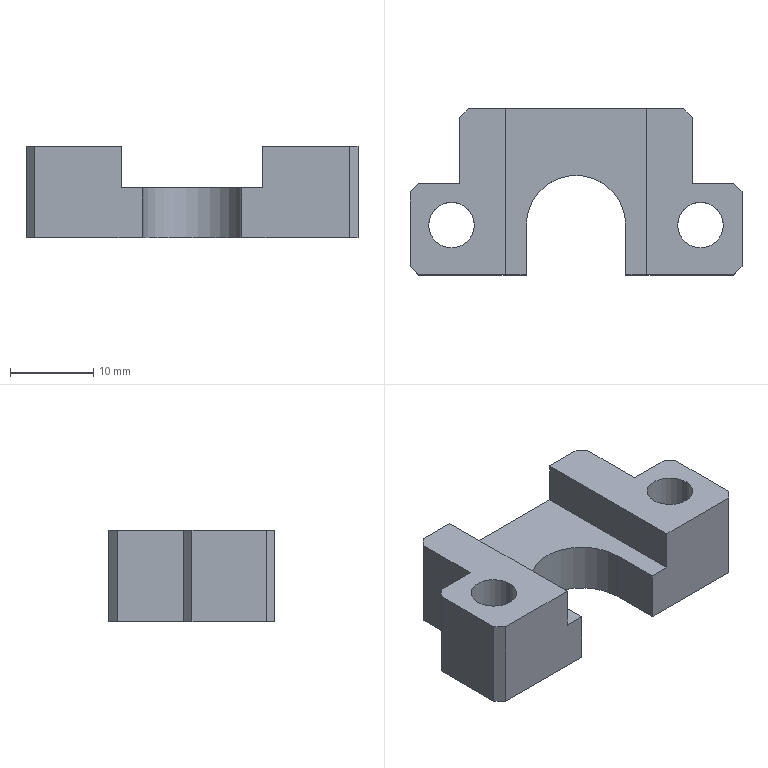Part | STEP file | union seat 11 | 1 solid | 28 faces | box 40 x 20 x 11 mm | volume 4585 mm3 | plane 23 | cylinder 5 | commonest cylinder face diameters 5.5 x4 12 x1